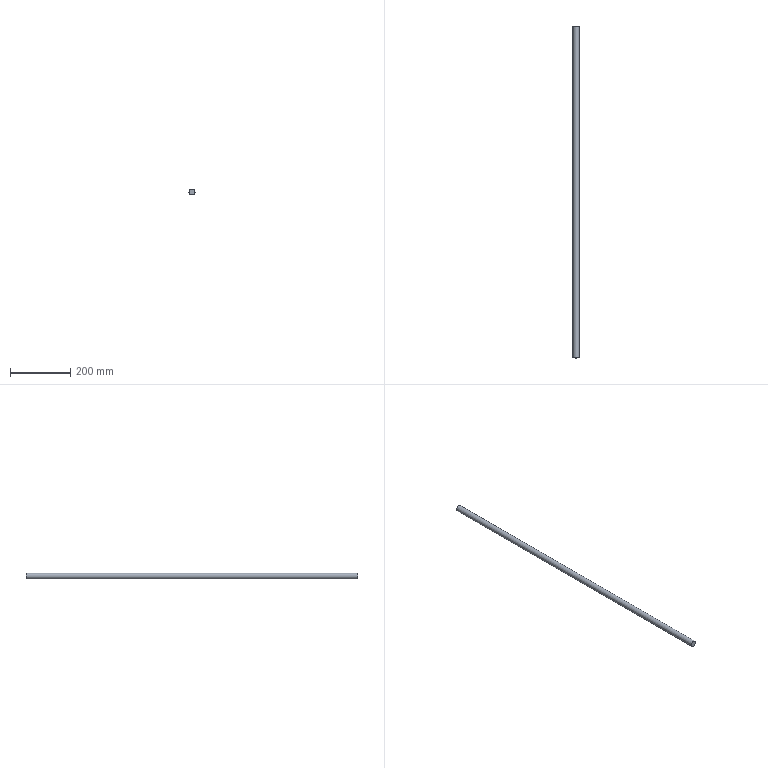Part | NX | features CYLINDER 1, DATUM_CSYS 1 | 1 solid | 3 faces | box 20 x 1100 x 20 mm | volume 345575 mm3 | plane 2 | cylinder 1 | commonest cylinder face diameters 20 x1
STEP:
#1=CARTESIAN_POINT('',(10.,-1100.,0.));
#2=VERTEX_POINT('',#1);
#3=CARTESIAN_POINT('',(0.,-1100.,0.));
#4=DIRECTION('',(0.,1.,0.));
#5=DIRECTION('',(1.,0.,0.));
#6=AXIS2_PLACEMENT_3D('',#3,#4,#5);
#7=CIRCLE('',#6,10.);
#8=EDGE_CURVE('',#2,#2,#7,.T.);
#9=ORIENTED_EDGE('',*,*,#8,.F.);
#10=EDGE_LOOP('',(#9));
#11=FACE_BOUND('',#10,.T.);
#12=CARTESIAN_POINT('',(0.,-1100.,0.));
#13=DIRECTION('',(0.,-1.,0.));
#14=DIRECTION('',(0.,0.,-1.));
#15=AXIS2_PLACEMENT_3D('',#12,#13,#14);
#16=PLANE('',#15);
#17=ADVANCED_FACE('',(#11),#16,.T.);
#18=CARTESIAN_POINT('',(10.,0.,0.));
#19=VERTEX_POINT('',#18);
#20=CARTESIAN_POINT('',(0.,0.,0.));
#21=DIRECTION('',(0.,-1.,0.));
#22=DIRECTION('',(1.,0.,0.));
#23=AXIS2_PLACEMENT_3D('',#20,#21,#22);
#24=CIRCLE('',#23,10.);
#25=EDGE_CURVE('',#19,#19,#24,.T.);
#26=ORIENTED_EDGE('',*,*,#25,.F.);
#27=EDGE_LOOP('',(#26));
#28=FACE_BOUND('',#27,.T.);
#29=CARTESIAN_POINT('',(0.,0.,0.));
#30=DIRECTION('',(0.,1.,0.));
#31=DIRECTION('',(0.,0.,1.));
#32=AXIS2_PLACEMENT_3D('',#29,#30,#31);
#33=PLANE('',#32);
#34=ADVANCED_FACE('',(#28),#33,.T.);
#35=ORIENTED_EDGE('',*,*,#8,.T.);
#36=EDGE_LOOP('',(#35));
#37=FACE_BOUND('',#36,.T.);
#38=ORIENTED_EDGE('',*,*,#25,.T.);
#39=EDGE_LOOP('',(#38));
#40=FACE_BOUND('',#39,.T.);
#41=CARTESIAN_POINT('',(0.,0.,0.));
#42=DIRECTION('',(0.,-1.,0.));
#43=DIRECTION('',(1.,0.,0.));
#44=AXIS2_PLACEMENT_3D('',#41,#42,#43);
#45=CYLINDRICAL_SURFACE('',#44,10.);
#46=ADVANCED_FACE('',(#37,#40),#45,.T.);
#47=CLOSED_SHELL('',(#17,#34,#46));
#48=MANIFOLD_SOLID_BREP('',#47);
#49=(LENGTH_UNIT()NAMED_UNIT(*)SI_UNIT(.MILLI.,.METRE.));
#50=UNCERTAINTY_MEASURE_WITH_UNIT(LENGTH_MEASURE(0.00001),#49,'','');
#51=(NAMED_UNIT(*)PLANE_ANGLE_UNIT()SI_UNIT($,.RADIAN.));
#52=(NAMED_UNIT(*)SI_UNIT($,.STERADIAN.)SOLID_ANGLE_UNIT());
#53=(GEOMETRIC_REPRESENTATION_CONTEXT(3)GLOBAL_UNCERTAINTY_ASSIGNED_CONTEXT((#50))GLOBAL_UNIT_ASSIGNED_CONTEXT((#49,#51,#52))REPRESENTATION_CONTEXT('',''));
#54=ADVANCED_BREP_SHAPE_REPRESENTATION('',(#48),#53);